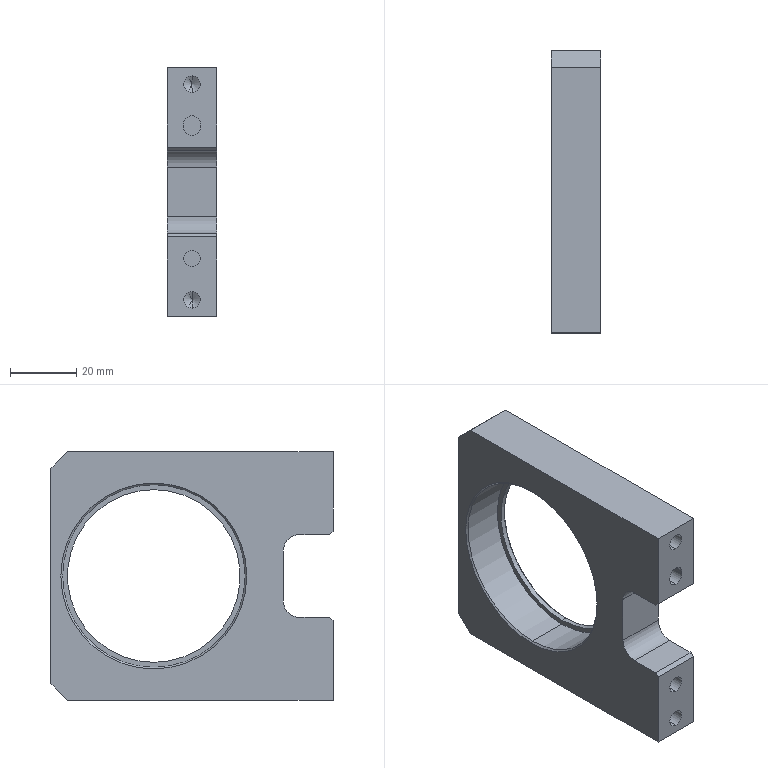Part | SolidWorks | features Chamfer 3, ICE 2, Extrusion 1, HoleWzd 1 | 1 solid | 42 faces | box 15 x 85 x 75 mm | volume 53244 mm3 | plane 19 | cylinder 15 | cone 8 | commonest cylinder face diameters 5 x9 10 x2 52 x2 55 x2
STEP:
#1=CARTESIAN_POINT('',(-7.,11.5,-27.5));
#2=VERTEX_POINT('',#1);
#3=CARTESIAN_POINT('',(-7.,11.5,27.5));
#4=VERTEX_POINT('',#3);
#5=CARTESIAN_POINT('',(-7.,11.5,0.));
#6=DIRECTION('',(-1.,0.,0.));
#7=DIRECTION('',(0.,0.,1.));
#8=AXIS2_PLACEMENT_3D('',#5,#6,#7);
#9=CIRCLE('',#8,27.5);
#10=EDGE_CURVE('',#2,#4,#9,.T.);
#11=ORIENTED_EDGE('',*,*,#10,.F.);
#12=CARTESIAN_POINT('',(-7.5,11.5,-28.));
#13=VERTEX_POINT('',#12);
#14=CARTESIAN_POINT('',(-7.5,11.5,-28.));
#15=DIRECTION('',(-0.7071,0.,-0.7071));
#16=VECTOR('',#15,1000.);
#17=LINE('',#14,#16);
#18=EDGE_CURVE('',#2,#13,#17,.T.);
#19=ORIENTED_EDGE('',*,*,#18,.T.);
#20=CARTESIAN_POINT('',(-7.5,11.5,28.));
#21=VERTEX_POINT('',#20);
#22=CARTESIAN_POINT('',(-7.5,11.5,0.));
#23=DIRECTION('',(1.,0.,0.));
#24=DIRECTION('',(0.,0.,1.));
#25=AXIS2_PLACEMENT_3D('',#22,#23,#24);
#26=CIRCLE('',#25,28.);
#27=EDGE_CURVE('',#21,#13,#26,.T.);
#28=ORIENTED_EDGE('',*,*,#27,.F.);
#29=CARTESIAN_POINT('',(-7.5,11.5,28.));
#30=DIRECTION('',(-0.7071,0.,0.7071));
#31=VECTOR('',#30,1000.);
#32=LINE('',#29,#31);
#33=EDGE_CURVE('',#4,#21,#32,.T.);
#34=ORIENTED_EDGE('',*,*,#33,.F.);
#35=EDGE_LOOP('',(#11,#19,#28,#34));
#36=FACE_OUTER_BOUND('',#35,.T.);
#37=CARTESIAN_POINT('',(-7.5,11.5,0.));
#38=DIRECTION('',(-1.,0.,0.));
#39=DIRECTION('',(0.,0.,1.));
#40=AXIS2_PLACEMENT_3D('',#37,#38,#39);
#41=CONICAL_SURFACE('',#40,28.,0.7854);
#42=ADVANCED_FACE('',(#36),#41,.F.);
#43=CARTESIAN_POINT('',(7.,11.5,26.));
#44=VERTEX_POINT('',#43);
#45=CARTESIAN_POINT('',(7.,11.5,-26.));
#46=VERTEX_POINT('',#45);
#47=CARTESIAN_POINT('',(7.,11.5,0.));
#48=DIRECTION('',(1.,0.,0.));
#49=DIRECTION('',(0.,0.,1.));
#50=AXIS2_PLACEMENT_3D('',#47,#48,#49);
#51=CIRCLE('',#50,26.);
#52=EDGE_CURVE('',#44,#46,#51,.T.);
#53=ORIENTED_EDGE('',*,*,#52,.F.);
#54=CARTESIAN_POINT('',(7.5,11.5,26.5));
#55=VERTEX_POINT('',#54);
#56=CARTESIAN_POINT('',(7.,11.5,26.));
#57=DIRECTION('',(0.7071,0.,0.7071));
#58=VECTOR('',#57,1000.);
#59=LINE('',#56,#58);
#60=EDGE_CURVE('',#44,#55,#59,.T.);
#61=ORIENTED_EDGE('',*,*,#60,.T.);
#62=CARTESIAN_POINT('',(7.5,11.5,-26.5));
#63=VERTEX_POINT('',#62);
#64=CARTESIAN_POINT('',(7.5,11.5,0.));
#65=DIRECTION('',(-1.,0.,0.));
#66=DIRECTION('',(0.,0.,1.));
#67=AXIS2_PLACEMENT_3D('',#64,#65,#66);
#68=CIRCLE('',#67,26.5);
#69=EDGE_CURVE('',#63,#55,#68,.T.);
#70=ORIENTED_EDGE('',*,*,#69,.F.);
#71=CARTESIAN_POINT('',(7.,11.5,-26.));
#72=DIRECTION('',(0.7071,0.,-0.7071));
#73=VECTOR('',#72,1000.);
#74=LINE('',#71,#73);
#75=EDGE_CURVE('',#46,#63,#74,.T.);
#76=ORIENTED_EDGE('',*,*,#75,.F.);
#77=EDGE_LOOP('',(#53,#61,#70,#76));
#78=FACE_OUTER_BOUND('',#77,.T.);
#79=CARTESIAN_POINT('',(7.,11.5,0.));
#80=DIRECTION('',(1.,0.,0.));
#81=DIRECTION('',(0.,0.,-1.));
#82=AXIS2_PLACEMENT_3D('',#79,#80,#81);
#83=CONICAL_SURFACE('',#82,26.,0.7854);
#84=ADVANCED_FACE('',(#78),#83,.F.);
#85=CARTESIAN_POINT('',(0.,-27.5,17.));
#86=VERTEX_POINT('',#85);
#87=CARTESIAN_POINT('',(2.5,-27.5,19.5));
#88=VERTEX_POINT('',#87);
#89=CARTESIAN_POINT('',(0.,-27.5,19.5));
#90=DIRECTION('',(0.,-1.,0.));
#91=DIRECTION('',(0.,0.,-1.));
#92=AXIS2_PLACEMENT_3D('',#89,#90,#91);
#93=CIRCLE('',#92,2.5);
#94=EDGE_CURVE('',#86,#88,#93,.T.);
#95=ORIENTED_EDGE('',*,*,#94,.F.);
#96=CARTESIAN_POINT('',(0.,-42.5,17.));
#97=VERTEX_POINT('',#96);
#98=CARTESIAN_POINT('',(0.,-27.5,17.));
#99=DIRECTION('',(0.,-1.,0.));
#100=VECTOR('',#99,1000.);
#101=LINE('',#98,#100);
#102=EDGE_CURVE('',#86,#97,#101,.T.);
#103=ORIENTED_EDGE('',*,*,#102,.T.);
#104=CARTESIAN_POINT('',(2.5,-42.5,19.5));
#105=VERTEX_POINT('',#104);
#106=CARTESIAN_POINT('',(0.,-42.5,19.5));
#107=DIRECTION('',(0.,-1.,0.));
#108=DIRECTION('',(0.,0.,-1.));
#109=AXIS2_PLACEMENT_3D('',#106,#107,#108);
#110=CIRCLE('',#109,2.5);
#111=EDGE_CURVE('',#97,#105,#110,.T.);
#112=ORIENTED_EDGE('',*,*,#111,.T.);
#113=CARTESIAN_POINT('',(2.5,-27.5,19.5));
#114=DIRECTION('',(0.,-1.,0.));
#115=VECTOR('',#114,1000.);
#116=LINE('',#113,#115);
#117=EDGE_CURVE('',#88,#105,#116,.T.);
#118=ORIENTED_EDGE('',*,*,#117,.F.);
#119=EDGE_LOOP('',(#95,#103,#112,#118));
#120=FACE_OUTER_BOUND('',#119,.T.);
#121=CARTESIAN_POINT('',(0.,-27.5,19.5));
#122=DIRECTION('',(0.,-1.,0.));
#123=DIRECTION('',(0.,0.,-1.));
#124=AXIS2_PLACEMENT_3D('',#121,#122,#123);
#125=CYLINDRICAL_SURFACE('',#124,2.5);
#126=ADVANCED_FACE('',(#120),#125,.F.);
#127=CARTESIAN_POINT('',(0.,-27.5,-17.5));
#128=VERTEX_POINT('',#127);
#129=CARTESIAN_POINT('',(0.,-27.5,-22.5));
#130=VERTEX_POINT('',#129);
#131=CARTESIAN_POINT('',(0.,-27.5,-20.));
#132=DIRECTION('',(0.,-1.,0.));
#133=DIRECTION('',(0.,0.,-1.));
#134=AXIS2_PLACEMENT_3D('',#131,#132,#133);
#135=CIRCLE('',#134,2.5);
#136=EDGE_CURVE('',#128,#130,#135,.T.);
#137=ORIENTED_EDGE('',*,*,#136,.F.);
#138=CARTESIAN_POINT('',(0.,-42.5,-17.5));
#139=VERTEX_POINT('',#138);
#140=CARTESIAN_POINT('',(0.,-27.5,-17.5));
#141=DIRECTION('',(0.,-1.,0.));
#142=VECTOR('',#141,1000.);
#143=LINE('',#140,#142);
#144=EDGE_CURVE('',#128,#139,#143,.T.);
#145=ORIENTED_EDGE('',*,*,#144,.T.);
#146=CARTESIAN_POINT('',(0.,-42.5,-22.5));
#147=VERTEX_POINT('',#146);
#148=CARTESIAN_POINT('',(0.,-42.5,-20.));
#149=DIRECTION('',(0.,-1.,0.));
#150=DIRECTION('',(0.,0.,-1.));
#151=AXIS2_PLACEMENT_3D('',#148,#149,#150);
#152=CIRCLE('',#151,2.5);
#153=EDGE_CURVE('',#139,#147,#152,.T.);
#154=ORIENTED_EDGE('',*,*,#153,.T.);
#155=CARTESIAN_POINT('',(0.,-27.5,-22.5));
#156=DIRECTION('',(0.,-1.,0.));
#157=VECTOR('',#156,1000.);
#158=LINE('',#155,#157);
#159=EDGE_CURVE('',#130,#147,#158,.T.);
#160=ORIENTED_EDGE('',*,*,#159,.F.);
#161=EDGE_LOOP('',(#137,#145,#154,#160));
#162=FACE_OUTER_BOUND('',#161,.T.);
#163=CARTESIAN_POINT('',(0.,-27.5,-20.));
#164=DIRECTION('',(0.,-1.,0.));
#165=DIRECTION('',(0.,0.,-1.));
#166=AXIS2_PLACEMENT_3D('',#163,#164,#165);
#167=CYLINDRICAL_SURFACE('',#166,2.5);
#168=ADVANCED_FACE('',(#162),#167,.F.);
#169=CARTESIAN_POINT('',(5.5,11.5,26.));
#170=VERTEX_POINT('',#169);
#171=CARTESIAN_POINT('',(5.5,11.5,-26.));
#172=VERTEX_POINT('',#171);
#173=CARTESIAN_POINT('',(5.5,11.5,0.));
#174=DIRECTION('',(1.,0.,0.));
#175=DIRECTION('',(0.,0.,-1.));
#176=AXIS2_PLACEMENT_3D('',#173,#174,#175);
#177=CIRCLE('',#176,26.);
#178=EDGE_CURVE('',#170,#172,#177,.T.);
#179=ORIENTED_EDGE('',*,*,#178,.F.);
#180=CARTESIAN_POINT('',(5.5,11.5,26.));
#181=DIRECTION('',(1.,0.,0.));
#182=VECTOR('',#181,1000.);
#183=LINE('',#180,#182);
#184=EDGE_CURVE('',#170,#44,#183,.T.);
#185=ORIENTED_EDGE('',*,*,#184,.T.);
#186=ORIENTED_EDGE('',*,*,#52,.T.);
#187=CARTESIAN_POINT('',(5.5,11.5,-26.));
#188=DIRECTION('',(1.,0.,0.));
#189=VECTOR('',#188,1000.);
#190=LINE('',#187,#189);
#191=EDGE_CURVE('',#172,#46,#190,.T.);
#192=ORIENTED_EDGE('',*,*,#191,.F.);
#193=EDGE_LOOP('',(#179,#185,#186,#192));
#194=FACE_OUTER_BOUND('',#193,.T.);
#195=CARTESIAN_POINT('',(5.5,11.5,0.));
#196=DIRECTION('',(1.,0.,0.));
#197=DIRECTION('',(0.,0.,-1.));
#198=AXIS2_PLACEMENT_3D('',#195,#196,#197);
#199=CYLINDRICAL_SURFACE('',#198,26.);
#200=ADVANCED_FACE('',(#194),#199,.F.);
#201=CARTESIAN_POINT('',(0.,-25.5,35.));
#202=VERTEX_POINT('',#201);
#203=CARTESIAN_POINT('',(0.,-25.5,30.));
#204=VERTEX_POINT('',#203);
#205=CARTESIAN_POINT('',(0.,-25.5,32.5));
#206=DIRECTION('',(0.,-1.,0.));
#207=DIRECTION('',(0.,0.,-1.));
#208=AXIS2_PLACEMENT_3D('',#205,#206,#207);
#209=CIRCLE('',#208,2.5);
#210=EDGE_CURVE('',#202,#204,#209,.T.);
#211=ORIENTED_EDGE('',*,*,#210,.F.);
#212=CARTESIAN_POINT('',(0.,-42.5,35.));
#213=VERTEX_POINT('',#212);
#214=CARTESIAN_POINT('',(0.,-42.5,35.));
#215=DIRECTION('',(0.,-1.,0.));
#216=VECTOR('',#215,1000.);
#217=LINE('',#214,#216);
#218=EDGE_CURVE('',#202,#213,#217,.T.);
#219=ORIENTED_EDGE('',*,*,#218,.T.);
#220=CARTESIAN_POINT('',(0.,-42.5,30.));
#221=VERTEX_POINT('',#220);
#222=CARTESIAN_POINT('',(0.,-42.5,32.5));
#223=DIRECTION('',(0.,-1.,0.));
#224=DIRECTION('',(0.,0.,-1.));
#225=AXIS2_PLACEMENT_3D('',#222,#223,#224);
#226=CIRCLE('',#225,2.5);
#227=EDGE_CURVE('',#213,#221,#226,.T.);
#228=ORIENTED_EDGE('',*,*,#227,.T.);
#229=CARTESIAN_POINT('',(0.,-42.5,30.));
#230=DIRECTION('',(0.,-1.,0.));
#231=VECTOR('',#230,1000.);
#232=LINE('',#229,#231);
#233=EDGE_CURVE('',#204,#221,#232,.T.);
#234=ORIENTED_EDGE('',*,*,#233,.F.);
#235=EDGE_LOOP('',(#211,#219,#228,#234));
#236=FACE_OUTER_BOUND('',#235,.T.);
#237=CARTESIAN_POINT('',(0.,-42.5,32.5));
#238=DIRECTION('',(0.,-1.,0.));
#239=DIRECTION('',(0.,0.,-1.));
#240=AXIS2_PLACEMENT_3D('',#237,#238,#239);
#241=CYLINDRICAL_SURFACE('',#240,2.5);
#242=ADVANCED_FACE('',(#236),#241,.F.);
#243=CARTESIAN_POINT('',(0.,-23.998,32.5));
#244=VERTEX_POINT('',#243);
#245=CARTESIAN_POINT('',(0.,-25.5,30.));
#246=DIRECTION('',(0.,-0.515,-0.8572));
#247=VECTOR('',#246,1000.);
#248=LINE('',#245,#247);
#249=EDGE_CURVE('',#244,#204,#248,.T.);
#250=ORIENTED_EDGE('',*,*,#249,.F.);
#251=CARTESIAN_POINT('',(0.,-25.5,35.));
#252=DIRECTION('',(0.,-0.515,0.8572));
#253=VECTOR('',#252,1000.);
#254=LINE('',#251,#253);
#255=EDGE_CURVE('',#244,#202,#254,.T.);
#256=ORIENTED_EDGE('',*,*,#255,.T.);
#257=ORIENTED_EDGE('',*,*,#210,.T.);
#258=EDGE_LOOP('',(#250,#256,#257));
#259=FACE_OUTER_BOUND('',#258,.T.);
#260=CARTESIAN_POINT('',(0.,-25.5,32.5));
#261=DIRECTION('',(0.,-1.,0.));
#262=DIRECTION('',(0.,0.,-1.));
#263=AXIS2_PLACEMENT_3D('',#260,#261,#262);
#264=CONICAL_SURFACE('',#263,2.5,1.03);
#265=ADVANCED_FACE('',(#259),#264,.F.);
#266=CARTESIAN_POINT('',(0.,-25.5,-30.));
#267=VERTEX_POINT('',#266);
#268=CARTESIAN_POINT('',(0.,-25.5,-35.));
#269=VERTEX_POINT('',#268);
#270=CARTESIAN_POINT('',(0.,-25.5,-32.5));
#271=DIRECTION('',(0.,-1.,0.));
#272=DIRECTION('',(0.,0.,-1.));
#273=AXIS2_PLACEMENT_3D('',#270,#271,#272);
#274=CIRCLE('',#273,2.5);
#275=EDGE_CURVE('',#267,#269,#274,.T.);
#276=ORIENTED_EDGE('',*,*,#275,.F.);
#277=CARTESIAN_POINT('',(0.,-42.5,-30.));
#278=VERTEX_POINT('',#277);
#279=CARTESIAN_POINT('',(0.,-42.5,-30.));
#280=DIRECTION('',(0.,-1.,0.));
#281=VECTOR('',#280,1000.);
#282=LINE('',#279,#281);
#283=EDGE_CURVE('',#267,#278,#282,.T.);
#284=ORIENTED_EDGE('',*,*,#283,.T.);
#285=CARTESIAN_POINT('',(0.,-42.5,-35.));
#286=VERTEX_POINT('',#285);
#287=CARTESIAN_POINT('',(0.,-42.5,-32.5));
#288=DIRECTION('',(0.,-1.,0.));
#289=DIRECTION('',(0.,0.,-1.));
#290=AXIS2_PLACEMENT_3D('',#287,#288,#289);
#291=CIRCLE('',#290,2.5);
#292=EDGE_CURVE('',#278,#286,#291,.T.);
#293=ORIENTED_EDGE('',*,*,#292,.T.);
#294=CARTESIAN_POINT('',(0.,-42.5,-35.));
#295=DIRECTION('',(0.,-1.,0.));
#296=VECTOR('',#295,1000.);
#297=LINE('',#294,#296);
#298=EDGE_CURVE('',#269,#286,#297,.T.);
#299=ORIENTED_EDGE('',*,*,#298,.F.);
#300=EDGE_LOOP('',(#276,#284,#293,#299));
#301=FACE_OUTER_BOUND('',#300,.T.);
#302=CARTESIAN_POINT('',(0.,-42.5,-32.5));
#303=DIRECTION('',(0.,-1.,0.));
#304=DIRECTION('',(0.,0.,-1.));
#305=AXIS2_PLACEMENT_3D('',#302,#303,#304);
#306=CYLINDRICAL_SURFACE('',#305,2.5);
#307=ADVANCED_FACE('',(#301),#306,.F.);
#308=CARTESIAN_POINT('',(0.,-23.998,-32.5));
#309=VERTEX_POINT('',#308);
#310=CARTESIAN_POINT('',(0.,-25.5,-35.));
#311=DIRECTION('',(0.,-0.515,-0.8572));
#312=VECTOR('',#311,1000.);
#313=LINE('',#310,#312);
#314=EDGE_CURVE('',#309,#269,#313,.T.);
#315=ORIENTED_EDGE('',*,*,#314,.F.);
#316=CARTESIAN_POINT('',(0.,-25.5,-30.));
#317=DIRECTION('',(0.,-0.515,0.8572));
#318=VECTOR('',#317,1000.);
#319=LINE('',#316,#318);
#320=EDGE_CURVE('',#309,#267,#319,.T.);
#321=ORIENTED_EDGE('',*,*,#320,.T.);
#322=ORIENTED_EDGE('',*,*,#275,.T.);
#323=EDGE_LOOP('',(#315,#321,#322));
#324=FACE_OUTER_BOUND('',#323,.T.);
#325=CARTESIAN_POINT('',(0.,-25.5,-32.5));
#326=DIRECTION('',(0.,-1.,0.));
#327=DIRECTION('',(0.,0.,-1.));
#328=AXIS2_PLACEMENT_3D('',#325,#326,#327);
#329=CONICAL_SURFACE('',#328,2.5,1.03);
#330=ADVANCED_FACE('',(#324),#329,.F.);
#331=CARTESIAN_POINT('',(5.5,11.5,27.5));
#332=VERTEX_POINT('',#331);
#333=CARTESIAN_POINT('',(5.5,11.5,-27.5));
#334=VERTEX_POINT('',#333);
#335=CARTESIAN_POINT('',(5.5,11.5,0.));
#336=DIRECTION('',(1.,0.,0.));
#337=DIRECTION('',(0.,0.,-1.));
#338=AXIS2_PLACEMENT_3D('',#335,#336,#337);
#339=CIRCLE('',#338,27.5);
#340=EDGE_CURVE('',#332,#334,#339,.T.);
#341=ORIENTED_EDGE('',*,*,#340,.T.);
#342=CARTESIAN_POINT('',(7.5,11.5,-27.5));
#343=DIRECTION('',(-1.,0.,0.));
#344=VECTOR('',#343,1000.);
#345=LINE('',#342,#344);
#346=EDGE_CURVE('',#334,#2,#345,.T.);
#347=ORIENTED_EDGE('',*,*,#346,.T.);
#348=ORIENTED_EDGE('',*,*,#10,.T.);
#349=CARTESIAN_POINT('',(7.5,11.5,27.5));
#350=DIRECTION('',(-1.,0.,0.));
#351=VECTOR('',#350,1000.);
#352=LINE('',#349,#351);
#353=EDGE_CURVE('',#332,#4,#352,.T.);
#354=ORIENTED_EDGE('',*,*,#353,.F.);
#355=EDGE_LOOP('',(#341,#347,#348,#354));
#356=FACE_OUTER_BOUND('',#355,.T.);
#357=CARTESIAN_POINT('',(7.5,11.5,0.));
#358=DIRECTION('',(-1.,0.,0.));
#359=DIRECTION('',(0.,0.,1.));
#360=AXIS2_PLACEMENT_3D('',#357,#358,#359);
#361=CYLINDRICAL_SURFACE('',#360,27.5);
#362=ADVANCED_FACE('',(#356),#361,.F.);
#363=ORIENTED_EDGE('',*,*,#346,.F.);
#364=CARTESIAN_POINT('',(5.5,11.5,0.));
#365=DIRECTION('',(1.,0.,0.));
#366=DIRECTION('',(0.,0.,-1.));
#367=AXIS2_PLACEMENT_3D('',#364,#365,#366);
#368=CIRCLE('',#367,27.5);
#369=EDGE_CURVE('',#334,#332,#368,.T.);
#370=ORIENTED_EDGE('',*,*,#369,.T.);
#371=ORIENTED_EDGE('',*,*,#353,.T.);
#372=CARTESIAN_POINT('',(-7.,11.5,0.));
#373=DIRECTION('',(-1.,0.,0.));
#374=DIRECTION('',(0.,0.,1.));
#375=AXIS2_PLACEMENT_3D('',#372,#373,#374);
#376=CIRCLE('',#375,27.5);
#377=EDGE_CURVE('',#4,#2,#376,.T.);
#378=ORIENTED_EDGE('',*,*,#377,.T.);
#379=EDGE_LOOP('',(#363,#370,#371,#378));
#380=FACE_OUTER_BOUND('',#379,.T.);
#381=CARTESIAN_POINT('',(7.5,11.5,0.));
#382=DIRECTION('',(-1.,0.,0.));
#383=DIRECTION('',(0.,0.,1.));
#384=AXIS2_PLACEMENT_3D('',#381,#382,#383);
#385=CYLINDRICAL_SURFACE('',#384,27.5);
#386=ADVANCED_FACE('',(#380),#385,.F.);
#387=ORIENTED_EDGE('',*,*,#69,.T.);
#388=CARTESIAN_POINT('',(7.5,11.5,0.));
#389=DIRECTION('',(-1.,0.,0.));
#390=DIRECTION('',(0.,0.,1.));
#391=AXIS2_PLACEMENT_3D('',#388,#389,#390);
#392=CIRCLE('',#391,26.5);
#393=EDGE_CURVE('',#55,#63,#392,.T.);
#394=ORIENTED_EDGE('',*,*,#393,.T.);
#395=EDGE_LOOP('',(#387,#394));
#396=FACE_BOUND('',#395,.T.);
#397=CARTESIAN_POINT('',(7.5,-42.5,37.5));
#398=VERTEX_POINT('',#397);
#399=CARTESIAN_POINT('',(7.5,-42.5,13.5));
#400=VERTEX_POINT('',#399);
#401=CARTESIAN_POINT('',(7.5,-42.5,37.5));
#402=DIRECTION('',(0.,0.,-1.));
#403=VECTOR('',#402,1000.);
#404=LINE('',#401,#403);
#405=EDGE_CURVE('',#398,#400,#404,.T.);
#406=ORIENTED_EDGE('',*,*,#405,.T.);
#407=CARTESIAN_POINT('',(7.5,-41.5,12.5));
#408=VERTEX_POINT('',#407);
#409=CARTESIAN_POINT('',(7.5,-41.5,12.5));
#410=DIRECTION('',(0.,0.7071,-0.7071));
#411=VECTOR('',#410,1000.);
#412=LINE('',#409,#411);
#413=EDGE_CURVE('',#400,#408,#412,.T.);
#414=ORIENTED_EDGE('',*,*,#413,.T.);
#415=CARTESIAN_POINT('',(7.5,-32.5,12.5));
#416=VERTEX_POINT('',#415);
#417=CARTESIAN_POINT('',(7.5,-42.5,12.5));
#418=DIRECTION('',(0.,1.,0.));
#419=VECTOR('',#418,1000.);
#420=LINE('',#417,#419);
#421=EDGE_CURVE('',#408,#416,#420,.T.);
#422=ORIENTED_EDGE('',*,*,#421,.T.);
#423=CARTESIAN_POINT('',(7.5,-27.5,7.5));
#424=VERTEX_POINT('',#423);
#425=CARTESIAN_POINT('',(7.5,-32.5,7.5));
#426=DIRECTION('',(-1.,0.,0.));
#427=DIRECTION('',(0.,0.,1.));
#428=AXIS2_PLACEMENT_3D('',#425,#426,#427);
#429=CIRCLE('',#428,5.);
#430=EDGE_CURVE('',#416,#424,#429,.T.);
#431=ORIENTED_EDGE('',*,*,#430,.T.);
#432=CARTESIAN_POINT('',(7.5,-27.5,-7.5));
#433=VERTEX_POINT('',#432);
#434=CARTESIAN_POINT('',(7.5,-27.5,7.5));
#435=DIRECTION('',(0.,0.,-1.));
#436=VECTOR('',#435,1000.);
#437=LINE('',#434,#436);
#438=EDGE_CURVE('',#424,#433,#437,.T.);
#439=ORIENTED_EDGE('',*,*,#438,.T.);
#440=CARTESIAN_POINT('',(7.5,-32.5,-12.5));
#441=VERTEX_POINT('',#440);
#442=CARTESIAN_POINT('',(7.5,-32.5,-7.5));
#443=DIRECTION('',(-1.,0.,0.));
#444=DIRECTION('',(0.,0.,1.));
#445=AXIS2_PLACEMENT_3D('',#442,#443,#444);
#446=CIRCLE('',#445,5.);
#447=EDGE_CURVE('',#433,#441,#446,.T.);
#448=ORIENTED_EDGE('',*,*,#447,.T.);
#449=CARTESIAN_POINT('',(7.5,-41.5,-12.5));
#450=VERTEX_POINT('',#449);
#451=CARTESIAN_POINT('',(7.5,-42.5,-12.5));
#452=DIRECTION('',(0.,-1.,0.));
#453=VECTOR('',#452,1000.);
#454=LINE('',#451,#453);
#455=EDGE_CURVE('',#441,#450,#454,.T.);
#456=ORIENTED_EDGE('',*,*,#455,.T.);
#457=CARTESIAN_POINT('',(7.5,-42.5,-13.5));
#458=VERTEX_POINT('',#457);
#459=CARTESIAN_POINT('',(7.5,-42.5,-13.5));
#460=DIRECTION('',(0.,-0.7071,-0.7071));
#461=VECTOR('',#460,1000.);
#462=LINE('',#459,#461);
#463=EDGE_CURVE('',#450,#458,#462,.T.);
#464=ORIENTED_EDGE('',*,*,#463,.T.);
#465=CARTESIAN_POINT('',(7.5,-42.5,-37.5));
#466=VERTEX_POINT('',#465);
#467=CARTESIAN_POINT('',(7.5,-42.5,-12.5));
#468=DIRECTION('',(0.,0.,-1.));
#469=VECTOR('',#468,1000.);
#470=LINE('',#467,#469);
#471=EDGE_CURVE('',#458,#466,#470,.T.);
#472=ORIENTED_EDGE('',*,*,#471,.T.);
#473=CARTESIAN_POINT('',(7.5,37.5,-37.5));
#474=VERTEX_POINT('',#473);
#475=CARTESIAN_POINT('',(7.5,-42.5,-37.5));
#476=DIRECTION('',(0.,1.,0.));
#477=VECTOR('',#476,1000.);
#478=LINE('',#475,#477);
#479=EDGE_CURVE('',#466,#474,#478,.T.);
#480=ORIENTED_EDGE('',*,*,#479,.T.);
#481=CARTESIAN_POINT('',(7.5,42.5,-32.5));
#482=VERTEX_POINT('',#481);
#483=CARTESIAN_POINT('',(7.5,42.5,-32.5));
#484=DIRECTION('',(0.,0.7071,0.7071));
#485=VECTOR('',#484,1000.);
#486=LINE('',#483,#485);
#487=EDGE_CURVE('',#474,#482,#486,.T.);
#488=ORIENTED_EDGE('',*,*,#487,.T.);
#489=CARTESIAN_POINT('',(7.5,42.5,32.5));
#490=VERTEX_POINT('',#489);
#491=CARTESIAN_POINT('',(7.5,42.5,37.5));
#492=DIRECTION('',(0.,0.,1.));
#493=VECTOR('',#492,1000.);
#494=LINE('',#491,#493);
#495=EDGE_CURVE('',#482,#490,#494,.T.);
#496=ORIENTED_EDGE('',*,*,#495,.T.);
#497=CARTESIAN_POINT('',(7.5,37.5,37.5));
#498=VERTEX_POINT('',#497);
#499=CARTESIAN_POINT('',(7.5,37.5,37.5));
#500=DIRECTION('',(0.,-0.7071,0.7071));
#501=VECTOR('',#500,1000.);
#502=LINE('',#499,#501);
#503=EDGE_CURVE('',#490,#498,#502,.T.);
#504=ORIENTED_EDGE('',*,*,#503,.T.);
#505=CARTESIAN_POINT('',(7.5,-42.5,37.5));
#506=DIRECTION('',(0.,-1.,0.));
#507=VECTOR('',#506,1000.);
#508=LINE('',#505,#507);
#509=EDGE_CURVE('',#498,#398,#508,.T.);
#510=ORIENTED_EDGE('',*,*,#509,.T.);
#511=EDGE_LOOP('',(#406,#414,#422,#431,#439,#448,#456,#464,#472,#480,#488,#496,#504,#510));
#512=FACE_OUTER_BOUND('',#511,.T.);
#513=CARTESIAN_POINT('',(7.5,-32.5,7.5));
#514=DIRECTION('',(-1.,0.,0.));
#515=DIRECTION('',(0.,0.,1.));
#516=AXIS2_PLACEMENT_3D('',#513,#514,#515);
#517=PLANE('',#516);
#518=ADVANCED_FACE('',(#396,#512),#517,.F.);
#519=ORIENTED_EDGE('',*,*,#27,.T.);
#520=CARTESIAN_POINT('',(-7.5,11.5,0.));
#521=DIRECTION('',(1.,0.,0.));
#522=DIRECTION('',(0.,0.,1.));
#523=AXIS2_PLACEMENT_3D('',#520,#521,#522);
#524=CIRCLE('',#523,28.);
#525=EDGE_CURVE('',#13,#21,#524,.T.);
#526=ORIENTED_EDGE('',*,*,#525,.T.);
#527=EDGE_LOOP('',(#519,#526));
#528=FACE_BOUND('',#527,.T.);
#529=CARTESIAN_POINT('',(-7.5,-41.5,12.5));
#530=VERTEX_POINT('',#529);
#531=CARTESIAN_POINT('',(-7.5,-32.5,12.5));
#532=VERTEX_POINT('',#531);
#533=CARTESIAN_POINT('',(-7.5,-42.5,12.5));
#534=DIRECTION('',(0.,1.,0.));
#535=VECTOR('',#534,1000.);
#536=LINE('',#533,#535);
#537=EDGE_CURVE('',#530,#532,#536,.T.);
#538=ORIENTED_EDGE('',*,*,#537,.F.);
#539=CARTESIAN_POINT('',(-7.5,-42.5,13.5));
#540=VERTEX_POINT('',#539);
#541=CARTESIAN_POINT('',(-7.5,-34.5,5.5));
#542=DIRECTION('',(0.,-0.7071,0.7071));
#543=VECTOR('',#542,1000.);
#544=LINE('',#541,#543);
#545=EDGE_CURVE('',#530,#540,#544,.T.);
#546=ORIENTED_EDGE('',*,*,#545,.T.);
#547=CARTESIAN_POINT('',(-7.5,-42.5,37.5));
#548=VERTEX_POINT('',#547);
#549=CARTESIAN_POINT('',(-7.5,-42.5,37.5));
#550=DIRECTION('',(0.,0.,-1.));
#551=VECTOR('',#550,1000.);
#552=LINE('',#549,#551);
#553=EDGE_CURVE('',#548,#540,#552,.T.);
#554=ORIENTED_EDGE('',*,*,#553,.F.);
#555=CARTESIAN_POINT('',(-7.5,37.5,37.5));
#556=VERTEX_POINT('',#555);
#557=CARTESIAN_POINT('',(-7.5,-42.5,37.5));
#558=DIRECTION('',(0.,-1.,0.));
#559=VECTOR('',#558,1000.);
#560=LINE('',#557,#559);
#561=EDGE_CURVE('',#556,#548,#560,.T.);
#562=ORIENTED_EDGE('',*,*,#561,.F.);
#563=CARTESIAN_POINT('',(-7.5,42.5,32.5));
#564=VERTEX_POINT('',#563);
#565=CARTESIAN_POINT('',(-7.5,17.5,57.5));
#566=DIRECTION('',(0.,0.7071,-0.7071));
#567=VECTOR('',#566,1000.);
#568=LINE('',#565,#567);
#569=EDGE_CURVE('',#556,#564,#568,.T.);
#570=ORIENTED_EDGE('',*,*,#569,.T.);
#571=CARTESIAN_POINT('',(-7.5,42.5,-32.5));
#572=VERTEX_POINT('',#571);
#573=CARTESIAN_POINT('',(-7.5,42.5,37.5));
#574=DIRECTION('',(0.,0.,1.));
#575=VECTOR('',#574,1000.);
#576=LINE('',#573,#575);
#577=EDGE_CURVE('',#572,#564,#576,.T.);
#578=ORIENTED_EDGE('',*,*,#577,.F.);
#579=CARTESIAN_POINT('',(-7.5,37.5,-37.5));
#580=VERTEX_POINT('',#579);
#581=CARTESIAN_POINT('',(-7.5,25.,-50.));
#582=DIRECTION('',(0.,-0.7071,-0.7071));
#583=VECTOR('',#582,1000.);
#584=LINE('',#581,#583);
#585=EDGE_CURVE('',#572,#580,#584,.T.);
#586=ORIENTED_EDGE('',*,*,#585,.T.);
#587=CARTESIAN_POINT('',(-7.5,-42.5,-37.5));
#588=VERTEX_POINT('',#587);
#589=CARTESIAN_POINT('',(-7.5,-42.5,-37.5));
#590=DIRECTION('',(0.,1.,0.));
#591=VECTOR('',#590,1000.);
#592=LINE('',#589,#591);
#593=EDGE_CURVE('',#588,#580,#592,.T.);
#594=ORIENTED_EDGE('',*,*,#593,.F.);
#595=CARTESIAN_POINT('',(-7.5,-42.5,-13.5));
#596=VERTEX_POINT('',#595);
#597=CARTESIAN_POINT('',(-7.5,-42.5,-12.5));
#598=DIRECTION('',(0.,0.,-1.));
#599=VECTOR('',#598,1000.);
#600=LINE('',#597,#599);
#601=EDGE_CURVE('',#596,#588,#600,.T.);
#602=ORIENTED_EDGE('',*,*,#601,.F.);
#603=CARTESIAN_POINT('',(-7.5,-41.5,-12.5));
#604=VERTEX_POINT('',#603);
#605=CARTESIAN_POINT('',(-7.5,-27.,2.));
#606=DIRECTION('',(0.,0.7071,0.7071));
#607=VECTOR('',#606,1000.);
#608=LINE('',#605,#607);
#609=EDGE_CURVE('',#596,#604,#608,.T.);
#610=ORIENTED_EDGE('',*,*,#609,.T.);
#611=CARTESIAN_POINT('',(-7.5,-32.5,-12.5));
#612=VERTEX_POINT('',#611);
#613=CARTESIAN_POINT('',(-7.5,-42.5,-12.5));
#614=DIRECTION('',(0.,-1.,0.));
#615=VECTOR('',#614,1000.);
#616=LINE('',#613,#615);
#617=EDGE_CURVE('',#612,#604,#616,.T.);
#618=ORIENTED_EDGE('',*,*,#617,.F.);
#619=CARTESIAN_POINT('',(-7.5,-27.5,-7.5));
#620=VERTEX_POINT('',#619);
#621=CARTESIAN_POINT('',(-7.5,-32.5,-7.5));
#622=DIRECTION('',(-1.,0.,0.));
#623=DIRECTION('',(0.,0.,1.));
#624=AXIS2_PLACEMENT_3D('',#621,#622,#623);
#625=CIRCLE('',#624,5.);
#626=EDGE_CURVE('',#620,#612,#625,.T.);
#627=ORIENTED_EDGE('',*,*,#626,.F.);
#628=CARTESIAN_POINT('',(-7.5,-27.5,7.5));
#629=VERTEX_POINT('',#628);
#630=CARTESIAN_POINT('',(-7.5,-27.5,7.5));
#631=DIRECTION('',(0.,0.,-1.));
#632=VECTOR('',#631,1000.);
#633=LINE('',#630,#632);
#634=EDGE_CURVE('',#629,#620,#633,.T.);
#635=ORIENTED_EDGE('',*,*,#634,.F.);
#636=CARTESIAN_POINT('',(-7.5,-32.5,7.5));
#637=DIRECTION('',(-1.,0.,0.));
#638=DIRECTION('',(0.,0.,1.));
#639=AXIS2_PLACEMENT_3D('',#636,#637,#638);
#640=CIRCLE('',#639,5.);
#641=EDGE_CURVE('',#532,#629,#640,.T.);
#642=ORIENTED_EDGE('',*,*,#641,.F.);
#643=EDGE_LOOP('',(#538,#546,#554,#562,#570,#578,#586,#594,#602,#610,#618,#627,#635,#642));
#644=FACE_OUTER_BOUND('',#643,.T.);
#645=CARTESIAN_POINT('',(-7.5,-32.5,7.5));
#646=DIRECTION('',(-1.,0.,0.));
#647=DIRECTION('',(0.,0.,1.));
#648=AXIS2_PLACEMENT_3D('',#645,#646,#647);
#649=PLANE('',#648);
#650=ADVANCED_FACE('',(#528,#644),#649,.T.);
#651=ORIENTED_EDGE('',*,*,#593,.T.);
#652=CARTESIAN_POINT('',(7.5,37.5,-37.5));
#653=DIRECTION('',(1.,0.,0.));
#654=VECTOR('',#653,1000.);
#655=LINE('',#652,#654);
#656=EDGE_CURVE('',#580,#474,#655,.T.);
#657=ORIENTED_EDGE('',*,*,#656,.T.);
#658=ORIENTED_EDGE('',*,*,#479,.F.);
#659=CARTESIAN_POINT('',(7.5,-42.5,-37.5));
#660=DIRECTION('',(-1.,0.,0.));
#661=VECTOR('',#660,1000.);
#662=LINE('',#659,#661);
#663=EDGE_CURVE('',#466,#588,#662,.T.);
#664=ORIENTED_EDGE('',*,*,#663,.T.);
#665=EDGE_LOOP('',(#651,#657,#658,#664));
#666=FACE_OUTER_BOUND('',#665,.T.);
#667=CARTESIAN_POINT('',(7.5,-42.5,-37.5));
#668=DIRECTION('',(0.,0.,1.));
#669=DIRECTION('',(1.,0.,0.));
#670=AXIS2_PLACEMENT_3D('',#667,#668,#669);
#671=PLANE('',#670);
#672=ADVANCED_FACE('',(#666),#671,.F.);
#673=ORIENTED_EDGE('',*,*,#495,.F.);
#674=CARTESIAN_POINT('',(7.5,42.5,-32.5));
#675=DIRECTION('',(-1.,0.,0.));
#676=VECTOR('',#675,1000.);
#677=LINE('',#674,#676);
#678=EDGE_CURVE('',#482,#572,#677,.T.);
#679=ORIENTED_EDGE('',*,*,#678,.T.);
#680=ORIENTED_EDGE('',*,*,#577,.T.);
#681=CARTESIAN_POINT('',(7.5,42.5,32.5));
#682=DIRECTION('',(1.,0.,0.));
#683=VECTOR('',#682,1000.);
#684=LINE('',#681,#683);
#685=EDGE_CURVE('',#564,#490,#684,.T.);
#686=ORIENTED_EDGE('',*,*,#685,.T.);
#687=EDGE_LOOP('',(#673,#679,#680,#686));
#688=FACE_OUTER_BOUND('',#687,.T.);
#689=CARTESIAN_POINT('',(7.5,42.5,37.5));
#690=DIRECTION('',(0.,-1.,0.));
#691=DIRECTION('',(0.,0.,-1.));
#692=AXIS2_PLACEMENT_3D('',#689,#690,#691);
#693=PLANE('',#692);
#694=ADVANCED_FACE('',(#688),#693,.F.);
#695=ORIENTED_EDGE('',*,*,#509,.F.);
#696=CARTESIAN_POINT('',(7.5,37.5,37.5));
#697=DIRECTION('',(-1.,0.,0.));
#698=VECTOR('',#697,1000.);
#699=LINE('',#696,#698);
#700=EDGE_CURVE('',#498,#556,#699,.T.);
#701=ORIENTED_EDGE('',*,*,#700,.T.);
#702=ORIENTED_EDGE('',*,*,#561,.T.);
#703=CARTESIAN_POINT('',(7.5,-42.5,37.5));
#704=DIRECTION('',(-1.,0.,0.));
#705=VECTOR('',#704,1000.);
#706=LINE('',#703,#705);
#707=EDGE_CURVE('',#398,#548,#706,.T.);
#708=ORIENTED_EDGE('',*,*,#707,.F.);
#709=EDGE_LOOP('',(#695,#701,#702,#708));
#710=FACE_OUTER_BOUND('',#709,.T.);
#711=CARTESIAN_POINT('',(7.5,-42.5,37.5));
#712=DIRECTION('',(0.,0.,-1.));
#713=DIRECTION('',(-1.,0.,0.));
#714=AXIS2_PLACEMENT_3D('',#711,#712,#713);
#715=PLANE('',#714);
#716=ADVANCED_FACE('',(#710),#715,.F.);
#717=CARTESIAN_POINT('',(-2.5,-42.5,20.5));
#718=VERTEX_POINT('',#717);
#719=CARTESIAN_POINT('',(-2.5,-42.5,19.5));
#720=VERTEX_POINT('',#719);
#721=CARTESIAN_POINT('',(-2.5,-42.5,20.5));
#722=DIRECTION('',(0.,0.,-1.));
#723=VECTOR('',#722,1000.);
#724=LINE('',#721,#723);
#725=EDGE_CURVE('',#718,#720,#724,.T.);
#726=ORIENTED_EDGE('',*,*,#725,.F.);
#727=CARTESIAN_POINT('',(2.5,-42.5,20.5));
#728=VERTEX_POINT('',#727);
#729=CARTESIAN_POINT('',(0.,-42.5,20.5));
#730=DIRECTION('',(0.,-1.,0.));
#731=DIRECTION('',(0.,0.,-1.));
#732=AXIS2_PLACEMENT_3D('',#729,#730,#731);
#733=CIRCLE('',#732,2.5);
#734=EDGE_CURVE('',#728,#718,#733,.T.);
#735=ORIENTED_EDGE('',*,*,#734,.F.);
#736=CARTESIAN_POINT('',(2.5,-42.5,20.5));
#737=DIRECTION('',(0.,0.,1.));
#738=VECTOR('',#737,1000.);
#739=LINE('',#736,#738);
#740=EDGE_CURVE('',#105,#728,#739,.T.);
#741=ORIENTED_EDGE('',*,*,#740,.F.);
#742=ORIENTED_EDGE('',*,*,#111,.F.);
#743=CARTESIAN_POINT('',(0.,-42.5,19.5));
#744=DIRECTION('',(0.,-1.,0.));
#745=DIRECTION('',(0.,0.,-1.));
#746=AXIS2_PLACEMENT_3D('',#743,#744,#745);
#747=CIRCLE('',#746,2.5);
#748=EDGE_CURVE('',#720,#97,#747,.T.);
#749=ORIENTED_EDGE('',*,*,#748,.F.);
#750=EDGE_LOOP('',(#726,#735,#741,#742,#749));
#751=FACE_BOUND('',#750,.T.);
#752=CARTESIAN_POINT('',(0.,-42.5,32.5));
#753=DIRECTION('',(0.,-1.,0.));
#754=DIRECTION('',(0.,0.,-1.));
#755=AXIS2_PLACEMENT_3D('',#752,#753,#754);
#756=CIRCLE('',#755,2.5);
#757=EDGE_CURVE('',#221,#213,#756,.T.);
#758=ORIENTED_EDGE('',*,*,#757,.F.);
#759=ORIENTED_EDGE('',*,*,#227,.F.);
#760=EDGE_LOOP('',(#758,#759));
#761=FACE_BOUND('',#760,.T.);
#762=ORIENTED_EDGE('',*,*,#553,.T.);
#763=CARTESIAN_POINT('',(7.5,-42.5,13.5));
#764=DIRECTION('',(1.,0.,0.));
#765=VECTOR('',#764,1000.);
#766=LINE('',#763,#765);
#767=EDGE_CURVE('',#540,#400,#766,.T.);
#768=ORIENTED_EDGE('',*,*,#767,.T.);
#769=ORIENTED_EDGE('',*,*,#405,.F.);
#770=ORIENTED_EDGE('',*,*,#707,.T.);
#771=EDGE_LOOP('',(#762,#768,#769,#770));
#772=FACE_OUTER_BOUND('',#771,.T.);
#773=CARTESIAN_POINT('',(7.5,-42.5,37.5));
#774=DIRECTION('',(0.,1.,0.));
#775=DIRECTION('',(0.,0.,1.));
#776=AXIS2_PLACEMENT_3D('',#773,#774,#775);
#777=PLANE('',#776);
#778=ADVANCED_FACE('',(#751,#761,#772),#777,.F.);
#779=ORIENTED_EDGE('',*,*,#421,.F.);
#780=CARTESIAN_POINT('',(7.5,-41.5,12.5));
#781=DIRECTION('',(-1.,0.,0.));
#782=VECTOR('',#781,1000.);
#783=LINE('',#780,#782);
#784=EDGE_CURVE('',#408,#530,#783,.T.);
#785=ORIENTED_EDGE('',*,*,#784,.T.);
#786=ORIENTED_EDGE('',*,*,#537,.T.);
#787=CARTESIAN_POINT('',(7.5,-32.5,12.5));
#788=DIRECTION('',(-1.,0.,0.));
#789=VECTOR('',#788,1000.);
#790=LINE('',#787,#789);
#791=EDGE_CURVE('',#416,#532,#790,.T.);
#792=ORIENTED_EDGE('',*,*,#791,.F.);
#793=EDGE_LOOP('',(#779,#785,#786,#792));
#794=FACE_OUTER_BOUND('',#793,.T.);
#795=CARTESIAN_POINT('',(7.5,-42.5,12.5));
#796=DIRECTION('',(0.,0.,1.));
#797=DIRECTION('',(1.,0.,0.));
#798=AXIS2_PLACEMENT_3D('',#795,#796,#797);
#799=PLANE('',#798);
#800=ADVANCED_FACE('',(#794),#799,.F.);
#801=ORIENTED_EDGE('',*,*,#641,.T.);
#802=CARTESIAN_POINT('',(7.5,-27.5,7.5));
#803=DIRECTION('',(-1.,0.,0.));
#804=VECTOR('',#803,1000.);
#805=LINE('',#802,#804);
#806=EDGE_CURVE('',#424,#629,#805,.T.);
#807=ORIENTED_EDGE('',*,*,#806,.F.);
#808=ORIENTED_EDGE('',*,*,#430,.F.);
#809=ORIENTED_EDGE('',*,*,#791,.T.);
#810=EDGE_LOOP('',(#801,#807,#808,#809));
#811=FACE_OUTER_BOUND('',#810,.T.);
#812=CARTESIAN_POINT('',(7.5,-32.5,7.5));
#813=DIRECTION('',(-1.,0.,0.));
#814=DIRECTION('',(0.,0.,1.));
#815=AXIS2_PLACEMENT_3D('',#812,#813,#814);
#816=CYLINDRICAL_SURFACE('',#815,5.);
#817=ADVANCED_FACE('',(#811),#816,.F.);
#818=ORIENTED_EDGE('',*,*,#634,.T.);
#819=CARTESIAN_POINT('',(7.5,-27.5,-7.5));
#820=DIRECTION('',(-1.,0.,0.));
#821=VECTOR('',#820,1000.);
#822=LINE('',#819,#821);
#823=EDGE_CURVE('',#433,#620,#822,.T.);
#824=ORIENTED_EDGE('',*,*,#823,.F.);
#825=ORIENTED_EDGE('',*,*,#438,.F.);
#826=ORIENTED_EDGE('',*,*,#806,.T.);
#827=EDGE_LOOP('',(#818,#824,#825,#826));
#828=FACE_OUTER_BOUND('',#827,.T.);
#829=CARTESIAN_POINT('',(7.5,-27.5,7.5));
#830=DIRECTION('',(0.,1.,0.));
#831=DIRECTION('',(0.,0.,1.));
#832=AXIS2_PLACEMENT_3D('',#829,#830,#831);
#833=PLANE('',#832);
#834=ADVANCED_FACE('',(#828),#833,.F.);
#835=ORIENTED_EDGE('',*,*,#626,.T.);
#836=CARTESIAN_POINT('',(7.5,-32.5,-12.5));
#837=DIRECTION('',(-1.,0.,0.));
#838=VECTOR('',#837,1000.);
#839=LINE('',#836,#838);
#840=EDGE_CURVE('',#441,#612,#839,.T.);
#841=ORIENTED_EDGE('',*,*,#840,.F.);
#842=ORIENTED_EDGE('',*,*,#447,.F.);
#843=ORIENTED_EDGE('',*,*,#823,.T.);
#844=EDGE_LOOP('',(#835,#841,#842,#843));
#845=FACE_OUTER_BOUND('',#844,.T.);
#846=CARTESIAN_POINT('',(7.5,-32.5,-7.5));
#847=DIRECTION('',(-1.,0.,0.));
#848=DIRECTION('',(0.,0.,1.));
#849=AXIS2_PLACEMENT_3D('',#846,#847,#848);
#850=CYLINDRICAL_SURFACE('',#849,5.);
#851=ADVANCED_FACE('',(#845),#850,.F.);
#852=ORIENTED_EDGE('',*,*,#617,.T.);
#853=CARTESIAN_POINT('',(7.5,-41.5,-12.5));
#854=DIRECTION('',(1.,0.,0.));
#855=VECTOR('',#854,1000.);
#856=LINE('',#853,#855);
#857=EDGE_CURVE('',#604,#450,#856,.T.);
#858=ORIENTED_EDGE('',*,*,#857,.T.);
#859=ORIENTED_EDGE('',*,*,#455,.F.);
#860=ORIENTED_EDGE('',*,*,#840,.T.);
#861=EDGE_LOOP('',(#852,#858,#859,#860));
#862=FACE_OUTER_BOUND('',#861,.T.);
#863=CARTESIAN_POINT('',(7.5,-42.5,-12.5));
#864=DIRECTION('',(0.,0.,-1.));
#865=DIRECTION('',(0.,1.,0.));
#866=AXIS2_PLACEMENT_3D('',#863,#864,#865);
#867=PLANE('',#866);
#868=ADVANCED_FACE('',(#862),#867,.F.);
#869=CARTESIAN_POINT('',(0.,-42.5,-20.));
#870=DIRECTION('',(0.,-1.,0.));
#871=DIRECTION('',(0.,0.,-1.));
#872=AXIS2_PLACEMENT_3D('',#869,#870,#871);
#873=CIRCLE('',#872,2.5);
#874=EDGE_CURVE('',#147,#139,#873,.T.);
#875=ORIENTED_EDGE('',*,*,#874,.F.);
#876=ORIENTED_EDGE('',*,*,#153,.F.);
#877=EDGE_LOOP('',(#875,#876));
#878=FACE_BOUND('',#877,.T.);
#879=CARTESIAN_POINT('',(0.,-42.5,-32.5));
#880=DIRECTION('',(0.,-1.,0.));
#881=DIRECTION('',(0.,0.,-1.));
#882=AXIS2_PLACEMENT_3D('',#879,#880,#881);
#883=CIRCLE('',#882,2.5);
#884=EDGE_CURVE('',#286,#278,#883,.T.);
#885=ORIENTED_EDGE('',*,*,#884,.F.);
#886=ORIENTED_EDGE('',*,*,#292,.F.);
#887=EDGE_LOOP('',(#885,#886));
#888=FACE_BOUND('',#887,.T.);
#889=ORIENTED_EDGE('',*,*,#471,.F.);
#890=CARTESIAN_POINT('',(7.5,-42.5,-13.5));
#891=DIRECTION('',(-1.,0.,0.));
#892=VECTOR('',#891,1000.);
#893=LINE('',#890,#892);
#894=EDGE_CURVE('',#458,#596,#893,.T.);
#895=ORIENTED_EDGE('',*,*,#894,.T.);
#896=ORIENTED_EDGE('',*,*,#601,.T.);
#897=ORIENTED_EDGE('',*,*,#663,.F.);
#898=EDGE_LOOP('',(#889,#895,#896,#897));
#899=FACE_OUTER_BOUND('',#898,.T.);
#900=CARTESIAN_POINT('',(7.5,-42.5,-12.5));
#901=DIRECTION('',(0.,1.,0.));
#902=DIRECTION('',(0.,0.,1.));
#903=AXIS2_PLACEMENT_3D('',#900,#901,#902);
#904=PLANE('',#903);
#905=ADVANCED_FACE('',(#878,#888,#899),#904,.F.);
#906=ORIENTED_EDGE('',*,*,#320,.F.);
#907=ORIENTED_EDGE('',*,*,#314,.T.);
#908=CARTESIAN_POINT('',(0.,-25.5,-32.5));
#909=DIRECTION('',(0.,-1.,0.));
#910=DIRECTION('',(0.,0.,-1.));
#911=AXIS2_PLACEMENT_3D('',#908,#909,#910);
#912=CIRCLE('',#911,2.5);
#913=EDGE_CURVE('',#269,#267,#912,.T.);
#914=ORIENTED_EDGE('',*,*,#913,.T.);
#915=EDGE_LOOP('',(#906,#907,#914));
#916=FACE_OUTER_BOUND('',#915,.T.);
#917=CARTESIAN_POINT('',(0.,-25.5,-32.5));
#918=DIRECTION('',(0.,-1.,0.));
#919=DIRECTION('',(0.,0.,-1.));
#920=AXIS2_PLACEMENT_3D('',#917,#918,#919);
#921=CONICAL_SURFACE('',#920,2.5,1.03);
#922=ADVANCED_FACE('',(#916),#921,.F.);
#923=ORIENTED_EDGE('',*,*,#283,.F.);
#924=ORIENTED_EDGE('',*,*,#913,.F.);
#925=ORIENTED_EDGE('',*,*,#298,.T.);
#926=ORIENTED_EDGE('',*,*,#884,.T.);
#927=EDGE_LOOP('',(#923,#924,#925,#926));
#928=FACE_OUTER_BOUND('',#927,.T.);
#929=CARTESIAN_POINT('',(0.,-42.5,-32.5));
#930=DIRECTION('',(0.,-1.,0.));
#931=DIRECTION('',(0.,0.,-1.));
#932=AXIS2_PLACEMENT_3D('',#929,#930,#931);
#933=CYLINDRICAL_SURFACE('',#932,2.5);
#934=ADVANCED_FACE('',(#928),#933,.F.);
#935=ORIENTED_EDGE('',*,*,#255,.F.);
#936=ORIENTED_EDGE('',*,*,#249,.T.);
#937=CARTESIAN_POINT('',(0.,-25.5,32.5));
#938=DIRECTION('',(0.,-1.,0.));
#939=DIRECTION('',(0.,0.,-1.));
#940=AXIS2_PLACEMENT_3D('',#937,#938,#939);
#941=CIRCLE('',#940,2.5);
#942=EDGE_CURVE('',#204,#202,#941,.T.);
#943=ORIENTED_EDGE('',*,*,#942,.T.);
#944=EDGE_LOOP('',(#935,#936,#943));
#945=FACE_OUTER_BOUND('',#944,.T.);
#946=CARTESIAN_POINT('',(0.,-25.5,32.5));
#947=DIRECTION('',(0.,-1.,0.));
#948=DIRECTION('',(0.,0.,-1.));
#949=AXIS2_PLACEMENT_3D('',#946,#947,#948);
#950=CONICAL_SURFACE('',#949,2.5,1.03);
#951=ADVANCED_FACE('',(#945),#950,.F.);
#952=ORIENTED_EDGE('',*,*,#218,.F.);
#953=ORIENTED_EDGE('',*,*,#942,.F.);
#954=ORIENTED_EDGE('',*,*,#233,.T.);
#955=ORIENTED_EDGE('',*,*,#757,.T.);
#956=EDGE_LOOP('',(#952,#953,#954,#955));
#957=FACE_OUTER_BOUND('',#956,.T.);
#958=CARTESIAN_POINT('',(0.,-42.5,32.5));
#959=DIRECTION('',(0.,-1.,0.));
#960=DIRECTION('',(0.,0.,-1.));
#961=AXIS2_PLACEMENT_3D('',#958,#959,#960);
#962=CYLINDRICAL_SURFACE('',#961,2.5);
#963=ADVANCED_FACE('',(#957),#962,.F.);
#964=CARTESIAN_POINT('',(5.5,11.5,0.));
#965=DIRECTION('',(1.,0.,0.));
#966=DIRECTION('',(0.,0.,-1.));
#967=AXIS2_PLACEMENT_3D('',#964,#965,#966);
#968=CIRCLE('',#967,26.);
#969=EDGE_CURVE('',#172,#170,#968,.T.);
#970=ORIENTED_EDGE('',*,*,#969,.T.);
#971=ORIENTED_EDGE('',*,*,#178,.T.);
#972=EDGE_LOOP('',(#970,#971));
#973=FACE_BOUND('',#972,.T.);
#974=ORIENTED_EDGE('',*,*,#340,.F.);
#975=ORIENTED_EDGE('',*,*,#369,.F.);
#976=EDGE_LOOP('',(#974,#975));
#977=FACE_OUTER_BOUND('',#976,.T.);
#978=CARTESIAN_POINT('',(5.5,11.5,0.));
#979=DIRECTION('',(1.,0.,0.));
#980=DIRECTION('',(0.,0.,-1.));
#981=AXIS2_PLACEMENT_3D('',#978,#979,#980);
#982=PLANE('',#981);
#983=ADVANCED_FACE('',(#973,#977),#982,.F.);
#984=ORIENTED_EDGE('',*,*,#184,.F.);
#985=ORIENTED_EDGE('',*,*,#969,.F.);
#986=ORIENTED_EDGE('',*,*,#191,.T.);
#987=CARTESIAN_POINT('',(7.,11.5,0.));
#988=DIRECTION('',(1.,0.,0.));
#989=DIRECTION('',(0.,0.,1.));
#990=AXIS2_PLACEMENT_3D('',#987,#988,#989);
#991=CIRCLE('',#990,26.);
#992=EDGE_CURVE('',#46,#44,#991,.T.);
#993=ORIENTED_EDGE('',*,*,#992,.T.);
#994=EDGE_LOOP('',(#984,#985,#986,#993));
#995=FACE_OUTER_BOUND('',#994,.T.);
#996=CARTESIAN_POINT('',(5.5,11.5,0.));
#997=DIRECTION('',(1.,0.,0.));
#998=DIRECTION('',(0.,0.,-1.));
#999=AXIS2_PLACEMENT_3D('',#996,#997,#998);
#1000=CYLINDRICAL_SURFACE('',#999,26.);
#1001=ADVANCED_FACE('',(#995),#1000,.F.);
#1002=ORIENTED_EDGE('',*,*,#487,.F.);
#1003=ORIENTED_EDGE('',*,*,#656,.F.);
#1004=ORIENTED_EDGE('',*,*,#585,.F.);
#1005=ORIENTED_EDGE('',*,*,#678,.F.);
#1006=EDGE_LOOP('',(#1002,#1003,#1004,#1005));
#1007=FACE_OUTER_BOUND('',#1006,.T.);
#1008=CARTESIAN_POINT('',(7.5,42.5,-32.5));
#1009=DIRECTION('',(0.,-0.7071,0.7071));
#1010=DIRECTION('',(-1.,0.,0.));
#1011=AXIS2_PLACEMENT_3D('',#1008,#1009,#1010);
#1012=PLANE('',#1011);
#1013=ADVANCED_FACE('',(#1007),#1012,.F.);
#1014=ORIENTED_EDGE('',*,*,#503,.F.);
#1015=ORIENTED_EDGE('',*,*,#685,.F.);
#1016=ORIENTED_EDGE('',*,*,#569,.F.);
#1017=ORIENTED_EDGE('',*,*,#700,.F.);
#1018=EDGE_LOOP('',(#1014,#1015,#1016,#1017));
#1019=FACE_OUTER_BOUND('',#1018,.T.);
#1020=CARTESIAN_POINT('',(7.5,37.5,37.5));
#1021=DIRECTION('',(0.,-0.7071,-0.7071));
#1022=DIRECTION('',(-1.,0.,0.));
#1023=AXIS2_PLACEMENT_3D('',#1020,#1021,#1022);
#1024=PLANE('',#1023);
#1025=ADVANCED_FACE('',(#1019),#1024,.F.);
#1026=ORIENTED_EDGE('',*,*,#144,.F.);
#1027=CARTESIAN_POINT('',(0.,-27.5,-20.));
#1028=DIRECTION('',(0.,-1.,0.));
#1029=DIRECTION('',(0.,0.,-1.));
#1030=AXIS2_PLACEMENT_3D('',#1027,#1028,#1029);
#1031=CIRCLE('',#1030,2.5);
#1032=EDGE_CURVE('',#130,#128,#1031,.T.);
#1033=ORIENTED_EDGE('',*,*,#1032,.F.);
#1034=ORIENTED_EDGE('',*,*,#159,.T.);
#1035=ORIENTED_EDGE('',*,*,#874,.T.);
#1036=EDGE_LOOP('',(#1026,#1033,#1034,#1035));
#1037=FACE_OUTER_BOUND('',#1036,.T.);
#1038=CARTESIAN_POINT('',(0.,-27.5,-20.));
#1039=DIRECTION('',(0.,-1.,0.));
#1040=DIRECTION('',(0.,0.,-1.));
#1041=AXIS2_PLACEMENT_3D('',#1038,#1039,#1040);
#1042=CYLINDRICAL_SURFACE('',#1041,2.5);
#1043=ADVANCED_FACE('',(#1037),#1042,.F.);
#1044=ORIENTED_EDGE('',*,*,#1032,.T.);
#1045=ORIENTED_EDGE('',*,*,#136,.T.);
#1046=EDGE_LOOP('',(#1044,#1045));
#1047=FACE_OUTER_BOUND('',#1046,.T.);
#1048=CARTESIAN_POINT('',(0.,-27.5,-20.));
#1049=DIRECTION('',(0.,-1.,0.));
#1050=DIRECTION('',(0.,0.,-1.));
#1051=AXIS2_PLACEMENT_3D('',#1048,#1049,#1050);
#1052=PLANE('',#1051);
#1053=ADVANCED_FACE('',(#1047),#1052,.T.);
#1054=ORIENTED_EDGE('',*,*,#734,.T.);
#1055=CARTESIAN_POINT('',(-2.5,-27.5,20.5));
#1056=VERTEX_POINT('',#1055);
#1057=CARTESIAN_POINT('',(-2.5,-27.5,20.5));
#1058=DIRECTION('',(0.,-1.,0.));
#1059=VECTOR('',#1058,1000.);
#1060=LINE('',#1057,#1059);
#1061=EDGE_CURVE('',#1056,#718,#1060,.T.);
#1062=ORIENTED_EDGE('',*,*,#1061,.F.);
#1063=CARTESIAN_POINT('',(2.5,-27.5,20.5));
#1064=VERTEX_POINT('',#1063);
#1065=CARTESIAN_POINT('',(0.,-27.5,20.5));
#1066=DIRECTION('',(0.,-1.,0.));
#1067=DIRECTION('',(0.,0.,-1.));
#1068=AXIS2_PLACEMENT_3D('',#1065,#1066,#1067);
#1069=CIRCLE('',#1068,2.5);
#1070=EDGE_CURVE('',#1064,#1056,#1069,.T.);
#1071=ORIENTED_EDGE('',*,*,#1070,.F.);
#1072=CARTESIAN_POINT('',(2.5,-27.5,20.5));
#1073=DIRECTION('',(0.,-1.,0.));
#1074=VECTOR('',#1073,1000.);
#1075=LINE('',#1072,#1074);
#1076=EDGE_CURVE('',#1064,#728,#1075,.T.);
#1077=ORIENTED_EDGE('',*,*,#1076,.T.);
#1078=EDGE_LOOP('',(#1054,#1062,#1071,#1077));
#1079=FACE_OUTER_BOUND('',#1078,.T.);
#1080=CARTESIAN_POINT('',(0.,-27.5,20.5));
#1081=DIRECTION('',(0.,-1.,0.));
#1082=DIRECTION('',(0.,0.,-1.));
#1083=AXIS2_PLACEMENT_3D('',#1080,#1081,#1082);
#1084=CYLINDRICAL_SURFACE('',#1083,2.5);
#1085=ADVANCED_FACE('',(#1079),#1084,.F.);
#1086=ORIENTED_EDGE('',*,*,#740,.T.);
#1087=ORIENTED_EDGE('',*,*,#1076,.F.);
#1088=CARTESIAN_POINT('',(2.5,-27.5,20.5));
#1089=DIRECTION('',(0.,0.,1.));
#1090=VECTOR('',#1089,1000.);
#1091=LINE('',#1088,#1090);
#1092=EDGE_CURVE('',#88,#1064,#1091,.T.);
#1093=ORIENTED_EDGE('',*,*,#1092,.F.);
#1094=ORIENTED_EDGE('',*,*,#117,.T.);
#1095=EDGE_LOOP('',(#1086,#1087,#1093,#1094));
#1096=FACE_OUTER_BOUND('',#1095,.T.);
#1097=CARTESIAN_POINT('',(2.5,-27.5,20.5));
#1098=DIRECTION('',(1.,0.,0.));
#1099=DIRECTION('',(0.,0.,-1.));
#1100=AXIS2_PLACEMENT_3D('',#1097,#1098,#1099);
#1101=PLANE('',#1100);
#1102=ADVANCED_FACE('',(#1096),#1101,.F.);
#1103=ORIENTED_EDGE('',*,*,#102,.F.);
#1104=CARTESIAN_POINT('',(-2.5,-27.5,19.5));
#1105=VERTEX_POINT('',#1104);
#1106=CARTESIAN_POINT('',(0.,-27.5,19.5));
#1107=DIRECTION('',(0.,-1.,0.));
#1108=DIRECTION('',(0.,0.,-1.));
#1109=AXIS2_PLACEMENT_3D('',#1106,#1107,#1108);
#1110=CIRCLE('',#1109,2.5);
#1111=EDGE_CURVE('',#1105,#86,#1110,.T.);
#1112=ORIENTED_EDGE('',*,*,#1111,.F.);
#1113=CARTESIAN_POINT('',(-2.5,-27.5,19.5));
#1114=DIRECTION('',(0.,-1.,0.));
#1115=VECTOR('',#1114,1000.);
#1116=LINE('',#1113,#1115);
#1117=EDGE_CURVE('',#1105,#720,#1116,.T.);
#1118=ORIENTED_EDGE('',*,*,#1117,.T.);
#1119=ORIENTED_EDGE('',*,*,#748,.T.);
#1120=EDGE_LOOP('',(#1103,#1112,#1118,#1119));
#1121=FACE_OUTER_BOUND('',#1120,.T.);
#1122=CARTESIAN_POINT('',(0.,-27.5,19.5));
#1123=DIRECTION('',(0.,-1.,0.));
#1124=DIRECTION('',(0.,0.,-1.));
#1125=AXIS2_PLACEMENT_3D('',#1122,#1123,#1124);
#1126=CYLINDRICAL_SURFACE('',#1125,2.5);
#1127=ADVANCED_FACE('',(#1121),#1126,.F.);
#1128=ORIENTED_EDGE('',*,*,#725,.T.);
#1129=ORIENTED_EDGE('',*,*,#1117,.F.);
#1130=CARTESIAN_POINT('',(-2.5,-27.5,20.5));
#1131=DIRECTION('',(0.,0.,-1.));
#1132=VECTOR('',#1131,1000.);
#1133=LINE('',#1130,#1132);
#1134=EDGE_CURVE('',#1056,#1105,#1133,.T.);
#1135=ORIENTED_EDGE('',*,*,#1134,.F.);
#1136=ORIENTED_EDGE('',*,*,#1061,.T.);
#1137=EDGE_LOOP('',(#1128,#1129,#1135,#1136));
#1138=FACE_OUTER_BOUND('',#1137,.T.);
#1139=CARTESIAN_POINT('',(-2.5,-27.5,20.5));
#1140=DIRECTION('',(-1.,0.,0.));
#1141=DIRECTION('',(0.,0.,1.));
#1142=AXIS2_PLACEMENT_3D('',#1139,#1140,#1141);
#1143=PLANE('',#1142);
#1144=ADVANCED_FACE('',(#1138),#1143,.F.);
#1145=ORIENTED_EDGE('',*,*,#1070,.T.);
#1146=ORIENTED_EDGE('',*,*,#1134,.T.);
#1147=ORIENTED_EDGE('',*,*,#1111,.T.);
#1148=ORIENTED_EDGE('',*,*,#94,.T.);
#1149=ORIENTED_EDGE('',*,*,#1092,.T.);
#1150=EDGE_LOOP('',(#1145,#1146,#1147,#1148,#1149));
#1151=FACE_OUTER_BOUND('',#1150,.T.);
#1152=CARTESIAN_POINT('',(0.,-27.5,20.5));
#1153=DIRECTION('',(0.,-1.,0.));
#1154=DIRECTION('',(0.,0.,-1.));
#1155=AXIS2_PLACEMENT_3D('',#1152,#1153,#1154);
#1156=PLANE('',#1155);
#1157=ADVANCED_FACE('',(#1151),#1156,.T.);
#1158=ORIENTED_EDGE('',*,*,#413,.F.);
#1159=ORIENTED_EDGE('',*,*,#767,.F.);
#1160=ORIENTED_EDGE('',*,*,#545,.F.);
#1161=ORIENTED_EDGE('',*,*,#784,.F.);
#1162=EDGE_LOOP('',(#1158,#1159,#1160,#1161));
#1163=FACE_OUTER_BOUND('',#1162,.T.);
#1164=CARTESIAN_POINT('',(7.5,-41.5,12.5));
#1165=DIRECTION('',(0.,0.7071,0.7071));
#1166=DIRECTION('',(-1.,0.,0.));
#1167=AXIS2_PLACEMENT_3D('',#1164,#1165,#1166);
#1168=PLANE('',#1167);
#1169=ADVANCED_FACE('',(#1163),#1168,.F.);
#1170=ORIENTED_EDGE('',*,*,#463,.F.);
#1171=ORIENTED_EDGE('',*,*,#857,.F.);
#1172=ORIENTED_EDGE('',*,*,#609,.F.);
#1173=ORIENTED_EDGE('',*,*,#894,.F.);
#1174=EDGE_LOOP('',(#1170,#1171,#1172,#1173));
#1175=FACE_OUTER_BOUND('',#1174,.T.);
#1176=CARTESIAN_POINT('',(7.5,-42.5,-13.5));
#1177=DIRECTION('',(0.,0.7071,-0.7071));
#1178=DIRECTION('',(-1.,0.,0.));
#1179=AXIS2_PLACEMENT_3D('',#1176,#1177,#1178);
#1180=PLANE('',#1179);
#1181=ADVANCED_FACE('',(#1175),#1180,.F.);
#1182=ORIENTED_EDGE('',*,*,#60,.F.);
#1183=ORIENTED_EDGE('',*,*,#992,.F.);
#1184=ORIENTED_EDGE('',*,*,#75,.T.);
#1185=ORIENTED_EDGE('',*,*,#393,.F.);
#1186=EDGE_LOOP('',(#1182,#1183,#1184,#1185));
#1187=FACE_OUTER_BOUND('',#1186,.T.);
#1188=CARTESIAN_POINT('',(7.,11.5,0.));
#1189=DIRECTION('',(1.,0.,0.));
#1190=DIRECTION('',(0.,0.,-1.));
#1191=AXIS2_PLACEMENT_3D('',#1188,#1189,#1190);
#1192=CONICAL_SURFACE('',#1191,26.,0.7854);
#1193=ADVANCED_FACE('',(#1187),#1192,.F.);
#1194=ORIENTED_EDGE('',*,*,#18,.F.);
#1195=ORIENTED_EDGE('',*,*,#377,.F.);
#1196=ORIENTED_EDGE('',*,*,#33,.T.);
#1197=ORIENTED_EDGE('',*,*,#525,.F.);
#1198=EDGE_LOOP('',(#1194,#1195,#1196,#1197));
#1199=FACE_OUTER_BOUND('',#1198,.T.);
#1200=CARTESIAN_POINT('',(-7.5,11.5,0.));
#1201=DIRECTION('',(-1.,0.,0.));
#1202=DIRECTION('',(0.,0.,1.));
#1203=AXIS2_PLACEMENT_3D('',#1200,#1201,#1202);
#1204=CONICAL_SURFACE('',#1203,28.,0.7854);
#1205=ADVANCED_FACE('',(#1199),#1204,.F.);
#1206=CLOSED_SHELL('',(#42,#84,#126,#168,#200,#242,#265,#307,#330,#362,#386,#518,#650,#672,#694,#716,#778,#800,#817,#834,#851,#868,#905,#922,#934,#951,#963,#983,#1001,#1013,#1025,#1043,#1053,#1085,#1102,#1127,#1144,#1157,#1169,#1181,#1193,#1205));
#1207=MANIFOLD_SOLID_BREP('',#1206);
#1208=CARTESIAN_POINT('',(0.,0.,0.));
#1209=DIRECTION('',(0.,0.,1.));
#1210=DIRECTION('',(1.,0.,0.));
#1211=AXIS2_PLACEMENT_3D('',#1208,#1209,#1210);
#1212=(LENGTH_UNIT()NAMED_UNIT(*)SI_UNIT(.MILLI.,.METRE.));
#1213=UNCERTAINTY_MEASURE_WITH_UNIT(LENGTH_MEASURE(0.00001),#1212,'','');
#1214=(NAMED_UNIT(*)PLANE_ANGLE_UNIT()SI_UNIT($,.RADIAN.));
#1215=(NAMED_UNIT(*)SI_UNIT($,.STERADIAN.)SOLID_ANGLE_UNIT());
#1216=(GEOMETRIC_REPRESENTATION_CONTEXT(3)GLOBAL_UNCERTAINTY_ASSIGNED_CONTEXT((#1213))GLOBAL_UNIT_ASSIGNED_CONTEXT((#1212,#1214,#1215))REPRESENTATION_CONTEXT('',''));
#1217=ADVANCED_BREP_SHAPE_REPRESENTATION('',(#1207,#1211),#1216);